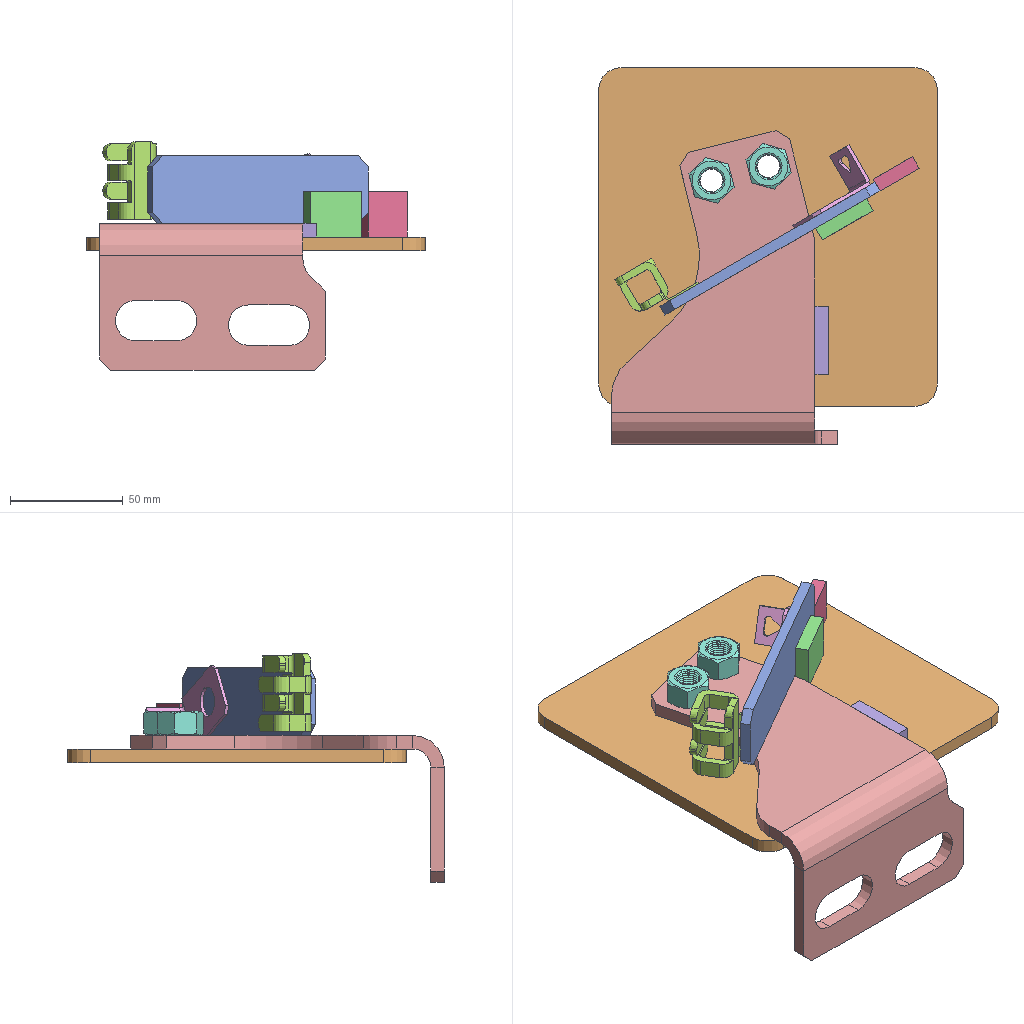Assembly | SolidWorks | 9 different items | 10 placed | box 150 x 167 x 101 mm
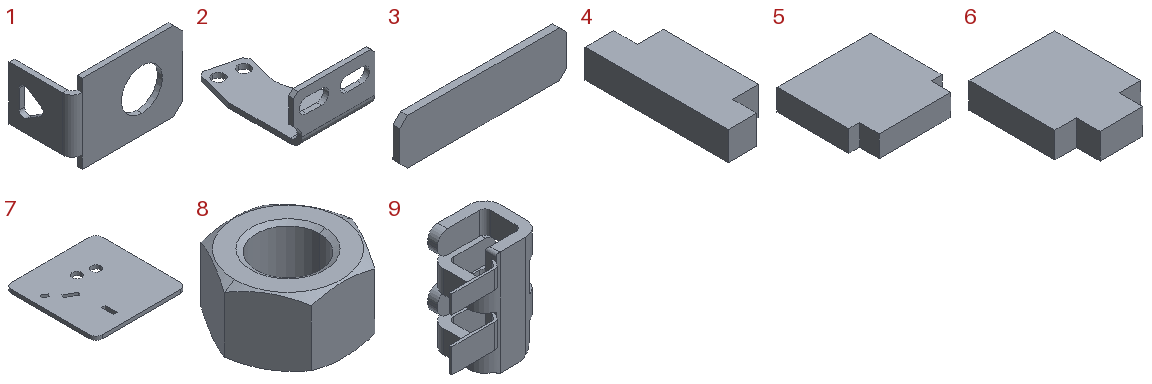Parts list (item | quantity | size | volume | features):
1 | x1 | 35 x 20 x 25 mm | 1534 mm3 | features ICE 2, Chamfer 1, FlatPattern 1, SMBaseFlange 1, SheetMetal 1
2 | x1 | 100 x 138.801 x 65 mm | 74939 mm3 | features ICE 2, Chamfer 1, Fillet 1, FlatPattern 1, SMBaseFlange 1, SheetMetal 1
3 | x1 | 110 x 4.5 x 30 mm | 14625 mm3 | features FlatPattern 1, SMBaseFlange 1, SheetMetal 1
4 | x1 | 11.5 x 30 x 6 mm | 1740 mm3 | features FlatPattern 1, SMBaseFlange 1, SheetMetal 1
5 | x1 | 26 x 25.5 x 6 mm | 3780 mm3 | features FlatPattern 1, SMBaseFlange 1, SheetMetal 1
6 | x1 | 20 x 25.5 x 6 mm | 2730 mm3 | features FlatPattern 1, SMBaseFlange 1, SheetMetal 1
7 | x1 | 150 x 150 x 6 mm | 130564 mm3 | features FlatPattern 1, SMBaseFlange 1, SheetMetal 1
8 | x2 | 27.713 x 24 x 14.8 mm | 5071 mm3 | features RevCut 2, Chamfer 1, Extrusion 1, LPattern 1
9 | x1 | 31.262 x 20.2 x 34.4 mm | 4311 mm3 | features MBimport 1
Mates (type | each side: item.copy, entity, surface, feature):
Coincident | 2.1 face plane Base-Flange1 | 3.1 face plane Base-Flange1
DistanceDim | 2.1 face plane Base-Flange1 | 3.1 edge | 3 times
Coincident | 3.1 face plane Base-Flange1 | 9.1 face plane 08036-D1630.STEP
DistanceDim | 9.1 face plane 08036-D1630.STEP | 3.1 face plane Base-Flange1 | 2 times
Coincident | 3.1 face plane Base-Flange1 | 1.1 face plane Base-Flange1
PlanarAngleDim | 1.1 face plane Base-Flange1 | 3.1 face plane Base-Flange1
DistanceDim | 1.1 face cylinder Cut-Extrude1 | 3.1 face plane Base-Flange1
DistanceDim | 3.1 face plane Base-Flange1 | 1.1 face cylinder Cut-Extrude1
Concentric | 2.1 face cylinder Cut-Extrude2 | 8.1 face cone EndChamfer
Coincident | 2.1 face plane Base-Flange1 | 8.1 face plane BaseNut
Concentric | 2.1 face cylinder Cut-Extrude2 | 8.2 face cone EndChamfer
Coincident | 2.1 face plane Base-Flange1 | 8.2 face plane BaseNut
Parallel | 2.1 face plane Cut-Extrude2 | 8.1 face plane BaseNut
Parallel | 2.1 face plane Cut-Extrude2 | 8.2 face plane BaseNut
InPlace | 2.1 face plane Base-Flange1 | 7.1 plane
InPlace | 2.1 face plane Cut-Extrude1 | 4.1 plane
InPlace | 7.1 face plane Base-Flange1 | 5.1 plane
InPlace | 7.1 face plane Base-Flange1 | 6.1 plane